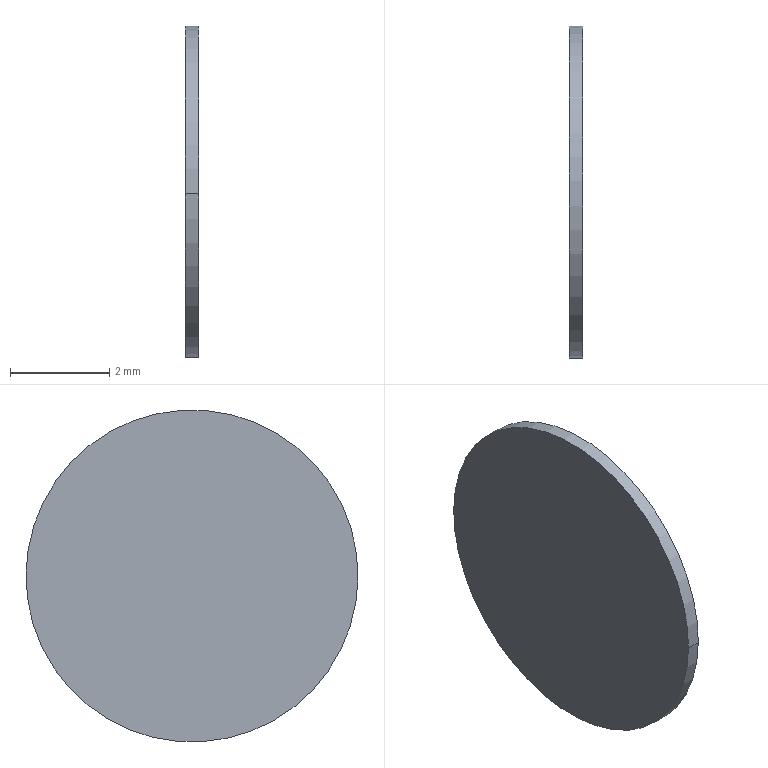Part | SolidWorks | features SplitBody 1 | 1 solid | 4 faces | box 0.2816 x 6.706 x 6.706 mm | volume 9.945 mm3 | cylinder 2 | plane 2 | commonest cylinder face diameters 6.706 x2
STEP:
#1=CARTESIAN_POINT('',(574.858,442.036,-342.519));
#2=VERTEX_POINT('',#1);
#3=CARTESIAN_POINT('',(574.858,448.741,-342.443));
#4=VERTEX_POINT('',#3);
#5=CARTESIAN_POINT('',(574.858,445.388,-342.481));
#6=DIRECTION('',(-1.,0.,0.));
#7=DIRECTION('',(0.,-0.9999,-0.01138));
#8=AXIS2_PLACEMENT_3D('',#5,#6,#7);
#9=CIRCLE('',#8,3.353);
#10=EDGE_CURVE('',#2,#4,#9,.T.);
#11=ORIENTED_EDGE('',*,*,#10,.F.);
#12=CARTESIAN_POINT('',(575.139,442.036,-342.519));
#13=VERTEX_POINT('',#12);
#14=CARTESIAN_POINT('',(574.858,442.036,-342.519));
#15=DIRECTION('',(1.,0.,0.));
#16=VECTOR('',#15,1000.);
#17=LINE('',#14,#16);
#18=EDGE_CURVE('',#2,#13,#17,.T.);
#19=ORIENTED_EDGE('',*,*,#18,.T.);
#20=CARTESIAN_POINT('',(575.139,448.741,-342.443));
#21=VERTEX_POINT('',#20);
#22=CARTESIAN_POINT('',(575.139,445.388,-342.481));
#23=DIRECTION('',(-1.,0.,0.));
#24=DIRECTION('',(0.,-0.9999,-0.01138));
#25=AXIS2_PLACEMENT_3D('',#22,#23,#24);
#26=CIRCLE('',#25,3.353);
#27=EDGE_CURVE('',#13,#21,#26,.T.);
#28=ORIENTED_EDGE('',*,*,#27,.T.);
#29=CARTESIAN_POINT('',(574.858,448.741,-342.443));
#30=DIRECTION('',(1.,0.,0.));
#31=VECTOR('',#30,1000.);
#32=LINE('',#29,#31);
#33=EDGE_CURVE('',#4,#21,#32,.T.);
#34=ORIENTED_EDGE('',*,*,#33,.F.);
#35=EDGE_LOOP('',(#11,#19,#28,#34));
#36=FACE_OUTER_BOUND('',#35,.T.);
#37=CARTESIAN_POINT('',(574.858,445.388,-342.481));
#38=DIRECTION('',(1.,0.,0.));
#39=DIRECTION('',(0.,0.9999,0.01138));
#40=AXIS2_PLACEMENT_3D('',#37,#38,#39);
#41=CYLINDRICAL_SURFACE('',#40,3.353);
#42=ADVANCED_FACE('',(#36),#41,.T.);
#43=ORIENTED_EDGE('',*,*,#18,.F.);
#44=CARTESIAN_POINT('',(574.858,445.388,-342.481));
#45=DIRECTION('',(-1.,0.,0.));
#46=DIRECTION('',(0.,-0.9999,-0.01138));
#47=AXIS2_PLACEMENT_3D('',#44,#45,#46);
#48=CIRCLE('',#47,3.353);
#49=EDGE_CURVE('',#4,#2,#48,.T.);
#50=ORIENTED_EDGE('',*,*,#49,.F.);
#51=ORIENTED_EDGE('',*,*,#33,.T.);
#52=CARTESIAN_POINT('',(575.139,445.388,-342.481));
#53=DIRECTION('',(-1.,0.,0.));
#54=DIRECTION('',(0.,-0.9999,-0.01138));
#55=AXIS2_PLACEMENT_3D('',#52,#53,#54);
#56=CIRCLE('',#55,3.353);
#57=EDGE_CURVE('',#21,#13,#56,.T.);
#58=ORIENTED_EDGE('',*,*,#57,.T.);
#59=EDGE_LOOP('',(#43,#50,#51,#58));
#60=FACE_OUTER_BOUND('',#59,.T.);
#61=CARTESIAN_POINT('',(574.858,445.388,-342.481));
#62=DIRECTION('',(1.,0.,0.));
#63=DIRECTION('',(0.,0.9999,0.01138));
#64=AXIS2_PLACEMENT_3D('',#61,#62,#63);
#65=CYLINDRICAL_SURFACE('',#64,3.353);
#66=ADVANCED_FACE('',(#60),#65,.T.);
#67=ORIENTED_EDGE('',*,*,#49,.T.);
#68=ORIENTED_EDGE('',*,*,#10,.T.);
#69=EDGE_LOOP('',(#67,#68));
#70=FACE_OUTER_BOUND('',#69,.T.);
#71=CARTESIAN_POINT('',(574.858,445.388,-342.481));
#72=DIRECTION('',(-1.,0.,0.));
#73=DIRECTION('',(0.,-0.9999,-0.01138));
#74=AXIS2_PLACEMENT_3D('',#71,#72,#73);
#75=PLANE('',#74);
#76=ADVANCED_FACE('',(#70),#75,.T.);
#77=ORIENTED_EDGE('',*,*,#57,.F.);
#78=ORIENTED_EDGE('',*,*,#27,.F.);
#79=EDGE_LOOP('',(#77,#78));
#80=FACE_OUTER_BOUND('',#79,.T.);
#81=CARTESIAN_POINT('',(575.139,445.388,-342.481));
#82=DIRECTION('',(-1.,0.,0.));
#83=DIRECTION('',(0.,-0.9999,-0.01138));
#84=AXIS2_PLACEMENT_3D('',#81,#82,#83);
#85=PLANE('',#84);
#86=ADVANCED_FACE('',(#80),#85,.F.);
#87=CLOSED_SHELL('',(#42,#66,#76,#86));
#88=MANIFOLD_SOLID_BREP('',#87);
#89=CARTESIAN_POINT('',(0.,0.,0.));
#90=DIRECTION('',(0.,0.,1.));
#91=DIRECTION('',(1.,0.,0.));
#92=AXIS2_PLACEMENT_3D('',#89,#90,#91);
#93=(LENGTH_UNIT()NAMED_UNIT(*)SI_UNIT(.MILLI.,.METRE.));
#94=UNCERTAINTY_MEASURE_WITH_UNIT(LENGTH_MEASURE(0.00001),#93,'','');
#95=(NAMED_UNIT(*)PLANE_ANGLE_UNIT()SI_UNIT($,.RADIAN.));
#96=(NAMED_UNIT(*)SI_UNIT($,.STERADIAN.)SOLID_ANGLE_UNIT());
#97=(GEOMETRIC_REPRESENTATION_CONTEXT(3)GLOBAL_UNCERTAINTY_ASSIGNED_CONTEXT((#94))GLOBAL_UNIT_ASSIGNED_CONTEXT((#93,#95,#96))REPRESENTATION_CONTEXT('',''));
#98=ADVANCED_BREP_SHAPE_REPRESENTATION('',(#88,#92),#97);